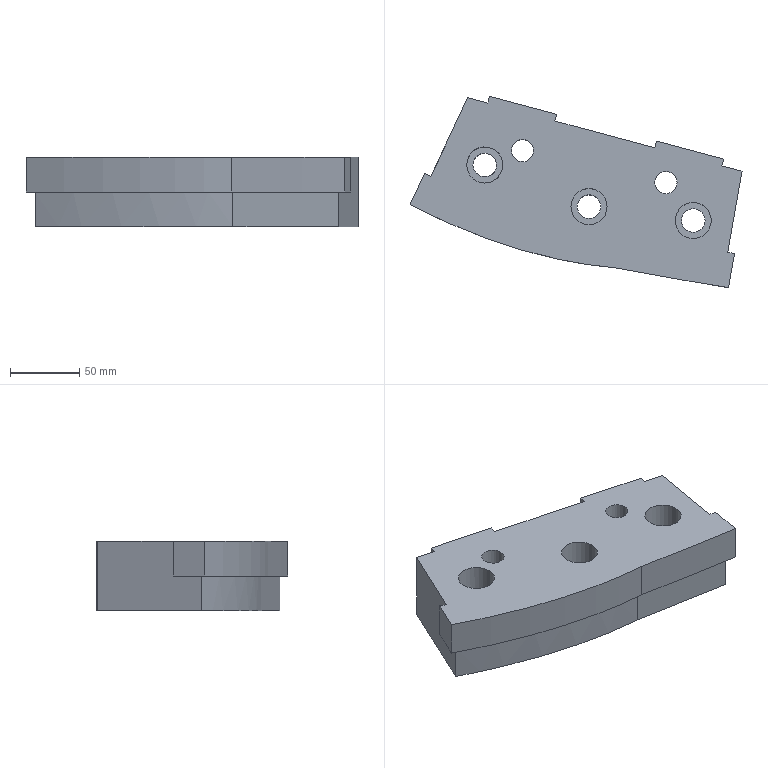Part | NX | features solid 2 | 1 solid | 33 faces | box 238.954 x 137.716 x 50 mm | volume 914448 mm3 | plane 21 | cylinder 8 | spline 4 | commonest cylinder face diameters 17 x3 26 x3 16 x2
STEP:
#1=CARTESIAN_POINT('',(-391.104,-138.3,0.));
#2=VERTEX_POINT('',#1);
#3=CARTESIAN_POINT('',(-376.615,-142.182,0.));
#4=VERTEX_POINT('',#3);
#5=CARTESIAN_POINT('',(-578.987,-87.957,0.));
#6=DIRECTION('',(0.9659,-0.2588,0.));
#7=VECTOR('',#6,1000.);
#8=LINE('',#5,#7);
#9=EDGE_CURVE('',#2,#4,#8,.T.);
#10=ORIENTED_EDGE('',*,*,#9,.T.);
#11=CARTESIAN_POINT('',(-376.615,-142.182,-50.));
#12=VERTEX_POINT('',#11);
#13=CARTESIAN_POINT('',(-376.615,-142.182,-50.));
#14=DIRECTION('',(0.,0.,-1.));
#15=VECTOR('',#14,1000.);
#16=LINE('',#13,#15);
#17=EDGE_CURVE('',#4,#12,#16,.T.);
#18=ORIENTED_EDGE('',*,*,#17,.T.);
#19=CARTESIAN_POINT('',(-391.104,-138.3,-50.));
#20=VERTEX_POINT('',#19);
#21=CARTESIAN_POINT('',(-578.987,-87.957,-50.));
#22=DIRECTION('',(0.9659,-0.2588,0.));
#23=VECTOR('',#22,1000.);
#24=LINE('',#21,#23);
#25=EDGE_CURVE('',#20,#12,#24,.T.);
#26=ORIENTED_EDGE('',*,*,#25,.F.);
#27=CARTESIAN_POINT('',(-391.104,-138.3,-50.));
#28=DIRECTION('',(0.,0.,1.));
#29=VECTOR('',#28,1000.);
#30=LINE('',#27,#29);
#31=EDGE_CURVE('',#20,#2,#30,.T.);
#32=ORIENTED_EDGE('',*,*,#31,.T.);
#33=EDGE_LOOP('',(#10,#18,#26,#32));
#34=FACE_BOUND('',#33,.T.);
#35=CARTESIAN_POINT('',(-578.987,-87.957,-50.));
#36=DIRECTION('',(-0.2588,-0.9659,0.));
#37=DIRECTION('',(0.9659,-0.2588,0.));
#38=AXIS2_PLACEMENT_3D('',#35,#36,#37);
#39=PLANE('',#38);
#40=ADVANCED_FACE('',(#34),#39,.F.);
#41=CARTESIAN_POINT('',(-381.983,-201.42,-25.));
#42=VERTEX_POINT('',#41);
#43=CARTESIAN_POINT('',(-386.907,-200.551,-25.));
#44=VERTEX_POINT('',#43);
#45=CARTESIAN_POINT('',(-377.059,-202.288,-25.));
#46=DIRECTION('',(-0.9848,0.1736,0.));
#47=VECTOR('',#46,1000.);
#48=LINE('',#45,#47);
#49=EDGE_CURVE('',#42,#44,#48,.T.);
#50=ORIENTED_EDGE('',*,*,#49,.F.);
#51=CARTESIAN_POINT('',(-386.325,-226.04,-25.));
#52=VERTEX_POINT('',#51);
#53=CARTESIAN_POINT('',(-386.325,-226.04,-25.));
#54=DIRECTION('',(-0.1736,-0.9848,0.));
#55=VECTOR('',#54,1000.);
#56=LINE('',#53,#55);
#57=EDGE_CURVE('',#42,#52,#56,.T.);
#58=ORIENTED_EDGE('',*,*,#57,.T.);
#59=CARTESIAN_POINT('',(-467.332,-211.778,-25.));
#60=VERTEX_POINT('',#59);
#61=CARTESIAN_POINT('',(-467.332,-211.778,-25.));
#62=CARTESIAN_POINT('',(-453.683,-214.296,-25.));
#63=CARTESIAN_POINT('',(-426.719,-219.268,-25.));
#64=CARTESIAN_POINT('',(-399.705,-223.975,-25.));
#65=CARTESIAN_POINT('',(-386.325,-226.04,-25.));
#66=B_SPLINE_CURVE_WITH_KNOTS('',3,(#61,#62,#63,#64,#65),.UNSPECIFIED.,.F.,.F.,(4,1,4),(0.6548,0.8295,1.),.UNSPECIFIED.);
#67=EDGE_CURVE('',#52,#60,#66,.F.);
#68=ORIENTED_EDGE('',*,*,#67,.T.);
#69=CARTESIAN_POINT('',(-615.57,-166.409,-25.));
#70=VERTEX_POINT('',#69);
#71=CARTESIAN_POINT('',(-615.57,-166.409,-25.));
#72=CARTESIAN_POINT('',(-612.933,-167.769,-25.));
#73=CARTESIAN_POINT('',(-595.69,-176.474,-25.));
#74=CARTESIAN_POINT('',(-562.946,-190.715,-25.));
#75=CARTESIAN_POINT('',(-515.99,-205.204,-25.));
#76=CARTESIAN_POINT('',(-483.626,-210.452,-25.));
#77=CARTESIAN_POINT('',(-467.332,-211.778,-25.));
#78=B_SPLINE_CURVE_WITH_KNOTS('',3,(#71,#72,#73,#74,#75,#76,#77),.UNSPECIFIED.,.F.,.F.,(4,1,1,1,4),(0.,0.03735,0.2432,0.449,0.6548),.UNSPECIFIED.);
#79=EDGE_CURVE('',#60,#70,#78,.F.);
#80=ORIENTED_EDGE('',*,*,#79,.T.);
#81=CARTESIAN_POINT('',(-605.004,-143.752,-25.));
#82=VERTEX_POINT('',#81);
#83=CARTESIAN_POINT('',(-615.57,-166.409,-25.));
#84=DIRECTION('',(-0.4226,-0.9063,0.));
#85=VECTOR('',#84,1000.);
#86=LINE('',#83,#85);
#87=EDGE_CURVE('',#82,#70,#86,.T.);
#88=ORIENTED_EDGE('',*,*,#87,.F.);
#89=CARTESIAN_POINT('',(-600.473,-145.865,-25.));
#90=VERTEX_POINT('',#89);
#91=CARTESIAN_POINT('',(-609.536,-141.638,-25.));
#92=DIRECTION('',(0.9063,-0.4226,0.));
#93=VECTOR('',#92,1000.);
#94=LINE('',#91,#93);
#95=EDGE_CURVE('',#82,#90,#94,.T.);
#96=ORIENTED_EDGE('',*,*,#95,.T.);
#97=CARTESIAN_POINT('',(-608.998,-164.148,-25.));
#98=VERTEX_POINT('',#97);
#99=CARTESIAN_POINT('',(-611.038,-168.522,-25.));
#100=DIRECTION('',(-0.4226,-0.9063,0.));
#101=VECTOR('',#100,1000.);
#102=LINE('',#99,#101);
#103=EDGE_CURVE('',#98,#90,#102,.F.);
#104=ORIENTED_EDGE('',*,*,#103,.F.);
#105=CARTESIAN_POINT('',(-466.674,-206.815,-25.));
#106=VERTEX_POINT('',#105);
#107=CARTESIAN_POINT('',(-608.998,-164.148,-25.));
#108=CARTESIAN_POINT('',(-597.84,-169.769,-25.));
#109=CARTESIAN_POINT('',(-575.112,-180.178,-25.));
#110=CARTESIAN_POINT('',(-545.758,-190.822,-25.));
#111=CARTESIAN_POINT('',(-521.796,-197.632,-25.));
#112=CARTESIAN_POINT('',(-503.595,-201.793,-25.));
#113=CARTESIAN_POINT('',(-488.289,-204.412,-25.));
#114=CARTESIAN_POINT('',(-475.931,-205.974,-25.));
#115=CARTESIAN_POINT('',(-469.818,-206.559,-25.));
#116=CARTESIAN_POINT('',(-466.674,-206.815,-25.));
#117=B_SPLINE_CURVE_WITH_KNOTS('',3,(#107,#108,#109,#110,#111,#112,#113,#114,#115,#116),.UNSPECIFIED.,.F.,.F.,(4,1,1,1,1,1,1,4),(0.03109,0.2737,0.5164,0.6377,0.759,0.8803,0.941,1.002),.UNSPECIFIED.);
#118=EDGE_CURVE('',#98,#106,#117,.T.);
#119=ORIENTED_EDGE('',*,*,#118,.T.);
#120=CARTESIAN_POINT('',(-390.397,-220.341,-25.));
#121=VERTEX_POINT('',#120);
#122=CARTESIAN_POINT('',(-466.674,-206.815,-25.));
#123=CARTESIAN_POINT('',(-453.956,-209.161,-25.));
#124=CARTESIAN_POINT('',(-428.53,-213.847,-25.));
#125=CARTESIAN_POINT('',(-403.113,-218.32,-25.));
#126=CARTESIAN_POINT('',(-390.397,-220.341,-25.));
#127=B_SPLINE_CURVE_WITH_KNOTS('',3,(#122,#123,#124,#125,#126),.UNSPECIFIED.,.F.,.F.,(4,1,4),(-0.003079,0.4686,0.9402),.UNSPECIFIED.);
#128=EDGE_CURVE('',#106,#121,#127,.T.);
#129=ORIENTED_EDGE('',*,*,#128,.T.);
#130=CARTESIAN_POINT('',(-391.249,-225.172,-25.));
#131=DIRECTION('',(-0.1736,-0.9848,0.));
#132=VECTOR('',#131,1000.);
#133=LINE('',#130,#132);
#134=EDGE_CURVE('',#121,#44,#133,.F.);
#135=ORIENTED_EDGE('',*,*,#134,.T.);
#136=EDGE_LOOP('',(#50,#58,#68,#80,#88,#96,#104,#119,#129,#135));
#137=FACE_BOUND('',#136,.T.);
#138=CARTESIAN_POINT('',(-280.448,-255.656,-25.));
#139=DIRECTION('',(0.,0.,-1.));
#140=DIRECTION('',(-1.,0.,0.));
#141=AXIS2_PLACEMENT_3D('',#138,#139,#140);
#142=PLANE('',#141);
#143=ADVANCED_FACE('',(#137),#142,.T.);
#144=CARTESIAN_POINT('',(-526.523,-127.421,0.));
#145=VERTEX_POINT('',#144);
#146=CARTESIAN_POINT('',(-534.523,-127.421,0.));
#147=DIRECTION('',(0.,0.,1.));
#148=DIRECTION('',(1.,0.,0.));
#149=AXIS2_PLACEMENT_3D('',#146,#147,#148);
#150=CIRCLE('',#149,8.);
#151=EDGE_CURVE('',#145,#145,#150,.T.);
#152=ORIENTED_EDGE('',*,*,#151,.F.);
#153=EDGE_LOOP('',(#152));
#154=FACE_BOUND('',#153,.T.);
#155=CARTESIAN_POINT('',(-423.374,-150.368,0.));
#156=VERTEX_POINT('',#155);
#157=CARTESIAN_POINT('',(-431.374,-150.368,0.));
#158=DIRECTION('',(0.,0.,1.));
#159=DIRECTION('',(1.,0.,0.));
#160=AXIS2_PLACEMENT_3D('',#157,#158,#159);
#161=CIRCLE('',#160,8.);
#162=EDGE_CURVE('',#156,#156,#161,.T.);
#163=ORIENTED_EDGE('',*,*,#162,.F.);
#164=EDGE_LOOP('',(#163));
#165=FACE_BOUND('',#164,.T.);
#166=CARTESIAN_POINT('',(-381.983,-201.42,0.));
#167=VERTEX_POINT('',#166);
#168=CARTESIAN_POINT('',(-386.907,-200.551,0.));
#169=VERTEX_POINT('',#168);
#170=CARTESIAN_POINT('',(-377.059,-202.288,0.));
#171=DIRECTION('',(-0.9848,0.1736,0.));
#172=VECTOR('',#171,1000.);
#173=LINE('',#170,#172);
#174=EDGE_CURVE('',#167,#169,#173,.T.);
#175=ORIENTED_EDGE('',*,*,#174,.T.);
#176=CARTESIAN_POINT('',(-391.249,-225.172,0.));
#177=DIRECTION('',(0.1736,0.9848,0.));
#178=VECTOR('',#177,1000.);
#179=LINE('',#176,#178);
#180=EDGE_CURVE('',#169,#4,#179,.T.);
#181=ORIENTED_EDGE('',*,*,#180,.T.);
#182=ORIENTED_EDGE('',*,*,#9,.F.);
#183=CARTESIAN_POINT('',(-389.81,-133.47,0.));
#184=VERTEX_POINT('',#183);
#185=CARTESIAN_POINT('',(-391.104,-138.3,0.));
#186=DIRECTION('',(0.2588,0.9659,0.));
#187=VECTOR('',#186,1000.);
#188=LINE('',#185,#187);
#189=EDGE_CURVE('',#2,#184,#188,.T.);
#190=ORIENTED_EDGE('',*,*,#189,.T.);
#191=CARTESIAN_POINT('',(-438.106,-120.529,0.));
#192=VERTEX_POINT('',#191);
#193=CARTESIAN_POINT('',(-577.693,-83.127,0.));
#194=DIRECTION('',(0.9659,-0.2588,0.));
#195=VECTOR('',#194,1000.);
#196=LINE('',#193,#195);
#197=EDGE_CURVE('',#192,#184,#196,.T.);
#198=ORIENTED_EDGE('',*,*,#197,.F.);
#199=CARTESIAN_POINT('',(-439.401,-125.359,0.));
#200=VERTEX_POINT('',#199);
#201=CARTESIAN_POINT('',(-439.401,-125.359,0.));
#202=DIRECTION('',(0.2588,0.9659,0.));
#203=VECTOR('',#202,1000.);
#204=LINE('',#201,#203);
#205=EDGE_CURVE('',#200,#192,#204,.T.);
#206=ORIENTED_EDGE('',*,*,#205,.F.);
#207=CARTESIAN_POINT('',(-511.297,-106.094,0.));
#208=VERTEX_POINT('',#207);
#209=CARTESIAN_POINT('',(-578.987,-87.957,0.));
#210=DIRECTION('',(0.9659,-0.2588,0.));
#211=VECTOR('',#210,1000.);
#212=LINE('',#209,#211);
#213=EDGE_CURVE('',#208,#200,#212,.T.);
#214=ORIENTED_EDGE('',*,*,#213,.F.);
#215=CARTESIAN_POINT('',(-510.003,-101.265,0.));
#216=VERTEX_POINT('',#215);
#217=CARTESIAN_POINT('',(-511.297,-106.094,0.));
#218=DIRECTION('',(0.2588,0.9659,0.));
#219=VECTOR('',#218,1000.);
#220=LINE('',#217,#219);
#221=EDGE_CURVE('',#208,#216,#220,.T.);
#222=ORIENTED_EDGE('',*,*,#221,.T.);
#223=CARTESIAN_POINT('',(-558.3,-88.324,0.));
#224=VERTEX_POINT('',#223);
#225=CARTESIAN_POINT('',(-712.375,-47.039,0.));
#226=DIRECTION('',(0.9659,-0.2588,0.));
#227=VECTOR('',#226,1000.);
#228=LINE('',#225,#227);
#229=EDGE_CURVE('',#224,#216,#228,.T.);
#230=ORIENTED_EDGE('',*,*,#229,.F.);
#231=CARTESIAN_POINT('',(-559.594,-93.153,0.));
#232=VERTEX_POINT('',#231);
#233=CARTESIAN_POINT('',(-559.594,-93.153,0.));
#234=DIRECTION('',(0.2588,0.9659,0.));
#235=VECTOR('',#234,1000.);
#236=LINE('',#233,#235);
#237=EDGE_CURVE('',#232,#224,#236,.T.);
#238=ORIENTED_EDGE('',*,*,#237,.F.);
#239=CARTESIAN_POINT('',(-574.083,-89.271,0.));
#240=VERTEX_POINT('',#239);
#241=CARTESIAN_POINT('',(-578.987,-87.957,0.));
#242=DIRECTION('',(0.9659,-0.2588,0.));
#243=VECTOR('',#242,1000.);
#244=LINE('',#241,#243);
#245=EDGE_CURVE('',#240,#232,#244,.T.);
#246=ORIENTED_EDGE('',*,*,#245,.F.);
#247=CARTESIAN_POINT('',(-600.473,-145.865,0.));
#248=VERTEX_POINT('',#247);
#249=CARTESIAN_POINT('',(-611.038,-168.522,0.));
#250=DIRECTION('',(0.4226,0.9063,0.));
#251=VECTOR('',#250,1000.);
#252=LINE('',#249,#251);
#253=EDGE_CURVE('',#248,#240,#252,.T.);
#254=ORIENTED_EDGE('',*,*,#253,.F.);
#255=CARTESIAN_POINT('',(-605.004,-143.752,0.));
#256=VERTEX_POINT('',#255);
#257=CARTESIAN_POINT('',(-609.536,-141.638,0.));
#258=DIRECTION('',(0.9063,-0.4226,0.));
#259=VECTOR('',#258,1000.);
#260=LINE('',#257,#259);
#261=EDGE_CURVE('',#256,#248,#260,.T.);
#262=ORIENTED_EDGE('',*,*,#261,.F.);
#263=CARTESIAN_POINT('',(-615.57,-166.409,0.));
#264=VERTEX_POINT('',#263);
#265=CARTESIAN_POINT('',(-615.57,-166.409,0.));
#266=DIRECTION('',(0.4226,0.9063,0.));
#267=VECTOR('',#266,1000.);
#268=LINE('',#265,#267);
#269=EDGE_CURVE('',#264,#256,#268,.T.);
#270=ORIENTED_EDGE('',*,*,#269,.F.);
#271=CARTESIAN_POINT('',(-467.332,-211.778,0.));
#272=VERTEX_POINT('',#271);
#273=CARTESIAN_POINT('',(-615.57,-166.409,0.));
#274=CARTESIAN_POINT('',(-612.933,-167.769,0.));
#275=CARTESIAN_POINT('',(-595.69,-176.474,0.));
#276=CARTESIAN_POINT('',(-562.946,-190.715,0.));
#277=CARTESIAN_POINT('',(-515.99,-205.204,0.));
#278=CARTESIAN_POINT('',(-483.626,-210.452,0.));
#279=CARTESIAN_POINT('',(-467.332,-211.778,0.));
#280=B_SPLINE_CURVE_WITH_KNOTS('',3,(#273,#274,#275,#276,#277,#278,#279),.UNSPECIFIED.,.F.,.F.,(4,1,1,1,4),(0.,0.03735,0.2432,0.449,0.6548),.UNSPECIFIED.);
#281=EDGE_CURVE('',#264,#272,#280,.T.);
#282=ORIENTED_EDGE('',*,*,#281,.T.);
#283=CARTESIAN_POINT('',(-386.325,-226.04,0.));
#284=VERTEX_POINT('',#283);
#285=CARTESIAN_POINT('',(-467.332,-211.778,0.));
#286=CARTESIAN_POINT('',(-453.683,-214.296,0.));
#287=CARTESIAN_POINT('',(-426.719,-219.268,0.));
#288=CARTESIAN_POINT('',(-399.705,-223.975,0.));
#289=CARTESIAN_POINT('',(-386.325,-226.04,0.));
#290=B_SPLINE_CURVE_WITH_KNOTS('',3,(#285,#286,#287,#288,#289),.UNSPECIFIED.,.F.,.F.,(4,1,4),(0.6548,0.8295,1.),.UNSPECIFIED.);
#291=EDGE_CURVE('',#272,#284,#290,.T.);
#292=ORIENTED_EDGE('',*,*,#291,.T.);
#293=CARTESIAN_POINT('',(-386.325,-226.04,0.));
#294=DIRECTION('',(0.1736,0.9848,0.));
#295=VECTOR('',#294,1000.);
#296=LINE('',#293,#295);
#297=EDGE_CURVE('',#284,#167,#296,.T.);
#298=ORIENTED_EDGE('',*,*,#297,.T.);
#299=EDGE_LOOP('',(#175,#181,#182,#190,#198,#206,#214,#222,#230,#238,#246,#254,#262,#270,#282,#292,#298));
#300=FACE_BOUND('',#299,.T.);
#301=CARTESIAN_POINT('',(-574.729,-137.741,0.));
#302=VERTEX_POINT('',#301);
#303=CARTESIAN_POINT('',(-561.729,-137.741,0.));
#304=DIRECTION('',(0.,0.,-1.));
#305=DIRECTION('',(-1.,0.,0.));
#306=AXIS2_PLACEMENT_3D('',#303,#304,#305);
#307=CIRCLE('',#306,13.);
#308=EDGE_CURVE('',#302,#302,#307,.T.);
#309=ORIENTED_EDGE('',*,*,#308,.T.);
#310=EDGE_LOOP('',(#309));
#311=FACE_BOUND('',#310,.T.);
#312=CARTESIAN_POINT('',(-499.729,-167.741,0.));
#313=VERTEX_POINT('',#312);
#314=CARTESIAN_POINT('',(-486.729,-167.741,0.));
#315=DIRECTION('',(0.,0.,-1.));
#316=DIRECTION('',(-1.,0.,0.));
#317=AXIS2_PLACEMENT_3D('',#314,#315,#316);
#318=CIRCLE('',#317,13.);
#319=EDGE_CURVE('',#313,#313,#318,.T.);
#320=ORIENTED_EDGE('',*,*,#319,.T.);
#321=EDGE_LOOP('',(#320));
#322=FACE_BOUND('',#321,.T.);
#323=CARTESIAN_POINT('',(-424.729,-177.741,0.));
#324=VERTEX_POINT('',#323);
#325=CARTESIAN_POINT('',(-411.729,-177.741,0.));
#326=DIRECTION('',(0.,0.,-1.));
#327=DIRECTION('',(-1.,0.,0.));
#328=AXIS2_PLACEMENT_3D('',#325,#326,#327);
#329=CIRCLE('',#328,13.);
#330=EDGE_CURVE('',#324,#324,#329,.T.);
#331=ORIENTED_EDGE('',*,*,#330,.T.);
#332=EDGE_LOOP('',(#331));
#333=FACE_BOUND('',#332,.T.);
#334=CARTESIAN_POINT('',(-488.834,-961.671,0.));
#335=DIRECTION('',(0.,0.,1.));
#336=DIRECTION('',(1.,0.,0.));
#337=AXIS2_PLACEMENT_3D('',#334,#335,#336);
#338=PLANE('',#337);
#339=ADVANCED_FACE('',(#154,#165,#300,#311,#322,#333),#338,.T.);
#340=CARTESIAN_POINT('',(-605.004,-143.752,-50.));
#341=DIRECTION('',(0.,0.,1.));
#342=VECTOR('',#341,1000.);
#343=LINE('',#340,#342);
#344=EDGE_CURVE('',#82,#256,#343,.T.);
#345=ORIENTED_EDGE('',*,*,#344,.F.);
#346=ORIENTED_EDGE('',*,*,#87,.T.);
#347=CARTESIAN_POINT('',(-615.57,-166.409,-50.));
#348=DIRECTION('',(0.,0.,1.));
#349=VECTOR('',#348,1000.);
#350=LINE('',#347,#349);
#351=EDGE_CURVE('',#70,#264,#350,.T.);
#352=ORIENTED_EDGE('',*,*,#351,.T.);
#353=ORIENTED_EDGE('',*,*,#269,.T.);
#354=EDGE_LOOP('',(#345,#346,#352,#353));
#355=FACE_BOUND('',#354,.T.);
#356=CARTESIAN_POINT('',(-615.57,-166.409,-50.));
#357=DIRECTION('',(0.9063,-0.4226,0.));
#358=DIRECTION('',(0.4226,0.9063,0.));
#359=AXIS2_PLACEMENT_3D('',#356,#357,#358);
#360=PLANE('',#359);
#361=ADVANCED_FACE('',(#355),#360,.F.);
#362=CARTESIAN_POINT('',(-526.523,-127.421,-50.));
#363=VERTEX_POINT('',#362);
#364=CARTESIAN_POINT('',(-534.523,-127.421,-50.));
#365=DIRECTION('',(0.,0.,1.));
#366=DIRECTION('',(1.,0.,0.));
#367=AXIS2_PLACEMENT_3D('',#364,#365,#366);
#368=CIRCLE('',#367,8.);
#369=EDGE_CURVE('',#363,#363,#368,.T.);
#370=ORIENTED_EDGE('',*,*,#369,.T.);
#371=EDGE_LOOP('',(#370));
#372=FACE_BOUND('',#371,.T.);
#373=CARTESIAN_POINT('',(-423.374,-150.368,-50.));
#374=VERTEX_POINT('',#373);
#375=CARTESIAN_POINT('',(-431.374,-150.368,-50.));
#376=DIRECTION('',(0.,0.,1.));
#377=DIRECTION('',(1.,0.,0.));
#378=AXIS2_PLACEMENT_3D('',#375,#376,#377);
#379=CIRCLE('',#378,8.);
#380=EDGE_CURVE('',#374,#374,#379,.T.);
#381=ORIENTED_EDGE('',*,*,#380,.T.);
#382=EDGE_LOOP('',(#381));
#383=FACE_BOUND('',#382,.T.);
#384=ORIENTED_EDGE('',*,*,#25,.T.);
#385=CARTESIAN_POINT('',(-390.397,-220.341,-50.));
#386=VERTEX_POINT('',#385);
#387=CARTESIAN_POINT('',(-391.297,-225.445,-50.));
#388=DIRECTION('',(0.1736,0.9848,0.));
#389=VECTOR('',#388,1000.);
#390=LINE('',#387,#389);
#391=EDGE_CURVE('',#386,#12,#390,.T.);
#392=ORIENTED_EDGE('',*,*,#391,.F.);
#393=CARTESIAN_POINT('',(-466.674,-206.815,-50.));
#394=VERTEX_POINT('',#393);
#395=CARTESIAN_POINT('',(-390.397,-220.341,-50.));
#396=CARTESIAN_POINT('',(-392.903,-219.943,-50.));
#397=CARTESIAN_POINT('',(-396.916,-219.29,-50.));
#398=CARTESIAN_POINT('',(-402.772,-218.308,-50.));
#399=CARTESIAN_POINT('',(-407.418,-217.517,-50.));
#400=CARTESIAN_POINT('',(-412.316,-216.67,-50.));
#401=CARTESIAN_POINT('',(-416.609,-215.918,-50.));
#402=CARTESIAN_POINT('',(-420.17,-215.288,-50.));
#403=CARTESIAN_POINT('',(-422.448,-214.883,-50.));
#404=CARTESIAN_POINT('',(-424.302,-214.553,-50.));
#405=CARTESIAN_POINT('',(-425.71,-214.301,-50.));
#406=CARTESIAN_POINT('',(-426.889,-214.089,-50.));
#407=CARTESIAN_POINT('',(-427.737,-213.937,-50.));
#408=CARTESIAN_POINT('',(-428.198,-213.854,-50.));
#409=CARTESIAN_POINT('',(-428.618,-213.778,-50.));
#410=CARTESIAN_POINT('',(-428.759,-213.753,-50.));
#411=CARTESIAN_POINT('',(-429.048,-213.701,-50.));
#412=CARTESIAN_POINT('',(-429.513,-213.617,-50.));
#413=CARTESIAN_POINT('',(-430.215,-213.49,-50.));
#414=CARTESIAN_POINT('',(-431.073,-213.335,-50.));
#415=CARTESIAN_POINT('',(-432.253,-213.122,-50.));
#416=CARTESIAN_POINT('',(-433.788,-212.844,-50.));
#417=CARTESIAN_POINT('',(-436.376,-212.374,-50.));
#418=CARTESIAN_POINT('',(-439.855,-211.74,-50.));
#419=CARTESIAN_POINT('',(-444.421,-210.906,-50.));
#420=CARTESIAN_POINT('',(-449.38,-209.997,-50.));
#421=CARTESIAN_POINT('',(-456.515,-208.687,-50.));
#422=CARTESIAN_POINT('',(-462.453,-207.593,-50.));
#423=CARTESIAN_POINT('',(-466.674,-206.815,-50.));
#424=B_SPLINE_CURVE_WITH_KNOTS('',3,(#395,#396,#397,#398,#399,#400,#401,#402,#403,#404,#405,#406,#407,#408,#409,#410,#411,#412,#413,#414,#415,#416,#417,#418,#419,#420,#421,#422,#423),.UNSPECIFIED.,.F.,.F.,(4,1,1,1,1,1,1,1,1,1,1,1,1,1,1,1,1,1,1,1,1,1,1,1,1,1,4),(0.,0.125,0.1875,0.25,0.3125,0.375,0.4062,0.4375,0.4531,0.4688,0.4844,0.4922,0.4961,0.5,0.5039,0.5078,0.5156,0.5312,0.5469,0.5625,0.5938,0.625,0.6875,0.75,0.8125,0.875,1.),.UNSPECIFIED.);
#425=EDGE_CURVE('',#394,#386,#424,.F.);
#426=ORIENTED_EDGE('',*,*,#425,.F.);
#427=CARTESIAN_POINT('',(-608.998,-164.148,-50.));
#428=VERTEX_POINT('',#427);
#429=CARTESIAN_POINT('',(-466.674,-206.815,-50.));
#430=CARTESIAN_POINT('',(-472.665,-206.327,-50.));
#431=CARTESIAN_POINT('',(-484.698,-204.994,-50.));
#432=CARTESIAN_POINT('',(-499.862,-202.433,-50.));
#433=CARTESIAN_POINT('',(-512.066,-199.847,-50.));
#434=CARTESIAN_POINT('',(-521.259,-197.639,-50.));
#435=CARTESIAN_POINT('',(-528.941,-195.578,-50.));
#436=CARTESIAN_POINT('',(-534.353,-194.012,-50.));
#437=CARTESIAN_POINT('',(-537.422,-193.092,-50.));
#438=CARTESIAN_POINT('',(-539.804,-192.361,-50.));
#439=CARTESIAN_POINT('',(-541.892,-191.707,-50.));
#440=CARTESIAN_POINT('',(-544.779,-190.785,-50.));
#441=CARTESIAN_POINT('',(-549.787,-189.14,-50.));
#442=CARTESIAN_POINT('',(-556.976,-186.647,-50.));
#443=CARTESIAN_POINT('',(-565.606,-183.442,-50.));
#444=CARTESIAN_POINT('',(-577.137,-178.882,-50.));
#445=CARTESIAN_POINT('',(-591.588,-172.642,-50.));
#446=CARTESIAN_POINT('',(-603.188,-167.075,-50.));
#447=CARTESIAN_POINT('',(-608.998,-164.148,-50.));
#448=B_SPLINE_CURVE_WITH_KNOTS('',3,(#429,#430,#431,#432,#433,#434,#435,#436,#437,#438,#439,#440,#441,#442,#443,#444,#445,#446,#447),.UNSPECIFIED.,.F.,.F.,(4,1,1,1,1,1,1,1,1,1,1,1,1,1,1,1,4),(0.,0.125,0.25,0.3125,0.375,0.4375,0.4688,0.4844,0.5,0.5156,0.5312,0.5625,0.625,0.6875,0.75,0.875,1.),.UNSPECIFIED.);
#449=EDGE_CURVE('',#428,#394,#448,.F.);
#450=ORIENTED_EDGE('',*,*,#449,.F.);
#451=CARTESIAN_POINT('',(-574.083,-89.271,-50.));
#452=VERTEX_POINT('',#451);
#453=CARTESIAN_POINT('',(-597.545,-139.587,-50.));
#454=DIRECTION('',(0.4226,0.9063,0.));
#455=VECTOR('',#454,1000.);
#456=LINE('',#453,#455);
#457=EDGE_CURVE('',#428,#452,#456,.T.);
#458=ORIENTED_EDGE('',*,*,#457,.T.);
#459=CARTESIAN_POINT('',(-559.594,-93.153,-50.));
#460=VERTEX_POINT('',#459);
#461=CARTESIAN_POINT('',(-578.987,-87.957,-50.));
#462=DIRECTION('',(0.9659,-0.2588,0.));
#463=VECTOR('',#462,1000.);
#464=LINE('',#461,#463);
#465=EDGE_CURVE('',#452,#460,#464,.T.);
#466=ORIENTED_EDGE('',*,*,#465,.T.);
#467=CARTESIAN_POINT('',(-558.3,-88.324,-50.));
#468=VERTEX_POINT('',#467);
#469=CARTESIAN_POINT('',(-559.594,-93.153,-50.));
#470=DIRECTION('',(0.2588,0.9659,0.));
#471=VECTOR('',#470,1000.);
#472=LINE('',#469,#471);
#473=EDGE_CURVE('',#460,#468,#472,.T.);
#474=ORIENTED_EDGE('',*,*,#473,.T.);
#475=CARTESIAN_POINT('',(-510.003,-101.265,-50.));
#476=VERTEX_POINT('',#475);
#477=CARTESIAN_POINT('',(-712.375,-47.039,-50.));
#478=DIRECTION('',(0.9659,-0.2588,0.));
#479=VECTOR('',#478,1000.);
#480=LINE('',#477,#479);
#481=EDGE_CURVE('',#468,#476,#480,.T.);
#482=ORIENTED_EDGE('',*,*,#481,.T.);
#483=CARTESIAN_POINT('',(-511.297,-106.094,-50.));
#484=VERTEX_POINT('',#483);
#485=CARTESIAN_POINT('',(-511.297,-106.094,-50.));
#486=DIRECTION('',(0.2588,0.9659,0.));
#487=VECTOR('',#486,1000.);
#488=LINE('',#485,#487);
#489=EDGE_CURVE('',#484,#476,#488,.T.);
#490=ORIENTED_EDGE('',*,*,#489,.F.);
#491=CARTESIAN_POINT('',(-439.401,-125.359,-50.));
#492=VERTEX_POINT('',#491);
#493=CARTESIAN_POINT('',(-578.987,-87.957,-50.));
#494=DIRECTION('',(0.9659,-0.2588,0.));
#495=VECTOR('',#494,1000.);
#496=LINE('',#493,#495);
#497=EDGE_CURVE('',#484,#492,#496,.T.);
#498=ORIENTED_EDGE('',*,*,#497,.T.);
#499=CARTESIAN_POINT('',(-438.106,-120.529,-50.));
#500=VERTEX_POINT('',#499);
#501=CARTESIAN_POINT('',(-439.401,-125.359,-50.));
#502=DIRECTION('',(0.2588,0.9659,0.));
#503=VECTOR('',#502,1000.);
#504=LINE('',#501,#503);
#505=EDGE_CURVE('',#492,#500,#504,.T.);
#506=ORIENTED_EDGE('',*,*,#505,.T.);
#507=CARTESIAN_POINT('',(-389.81,-133.47,-50.));
#508=VERTEX_POINT('',#507);
#509=CARTESIAN_POINT('',(-577.693,-83.127,-50.));
#510=DIRECTION('',(0.9659,-0.2588,0.));
#511=VECTOR('',#510,1000.);
#512=LINE('',#509,#511);
#513=EDGE_CURVE('',#500,#508,#512,.T.);
#514=ORIENTED_EDGE('',*,*,#513,.T.);
#515=CARTESIAN_POINT('',(-391.104,-138.3,-50.));
#516=DIRECTION('',(0.2588,0.9659,0.));
#517=VECTOR('',#516,1000.);
#518=LINE('',#515,#517);
#519=EDGE_CURVE('',#20,#508,#518,.T.);
#520=ORIENTED_EDGE('',*,*,#519,.F.);
#521=EDGE_LOOP('',(#384,#392,#426,#450,#458,#466,#474,#482,#490,#498,#506,#514,#520));
#522=FACE_BOUND('',#521,.T.);
#523=CARTESIAN_POINT('',(-420.229,-177.741,-50.));
#524=VERTEX_POINT('',#523);
#525=CARTESIAN_POINT('',(-411.729,-177.741,-50.));
#526=DIRECTION('',(0.,0.,-1.));
#527=DIRECTION('',(-1.,0.,0.));
#528=AXIS2_PLACEMENT_3D('',#525,#526,#527);
#529=CIRCLE('',#528,8.5);
#530=EDGE_CURVE('',#524,#524,#529,.T.);
#531=ORIENTED_EDGE('',*,*,#530,.F.);
#532=EDGE_LOOP('',(#531));
#533=FACE_BOUND('',#532,.T.);
#534=CARTESIAN_POINT('',(-495.229,-167.741,-50.));
#535=VERTEX_POINT('',#534);
#536=CARTESIAN_POINT('',(-486.729,-167.741,-50.));
#537=DIRECTION('',(0.,0.,-1.));
#538=DIRECTION('',(-1.,0.,0.));
#539=AXIS2_PLACEMENT_3D('',#536,#537,#538);
#540=CIRCLE('',#539,8.5);
#541=EDGE_CURVE('',#535,#535,#540,.T.);
#542=ORIENTED_EDGE('',*,*,#541,.F.);
#543=EDGE_LOOP('',(#542));
#544=FACE_BOUND('',#543,.T.);
#545=CARTESIAN_POINT('',(-570.229,-137.741,-50.));
#546=VERTEX_POINT('',#545);
#547=CARTESIAN_POINT('',(-561.729,-137.741,-50.));
#548=DIRECTION('',(0.,0.,-1.));
#549=DIRECTION('',(-1.,0.,0.));
#550=AXIS2_PLACEMENT_3D('',#547,#548,#549);
#551=CIRCLE('',#550,8.5);
#552=EDGE_CURVE('',#546,#546,#551,.T.);
#553=ORIENTED_EDGE('',*,*,#552,.F.);
#554=EDGE_LOOP('',(#553));
#555=FACE_BOUND('',#554,.T.);
#556=CARTESIAN_POINT('',(-488.834,-961.671,-50.));
#557=DIRECTION('',(0.,0.,1.));
#558=DIRECTION('',(1.,0.,0.));
#559=AXIS2_PLACEMENT_3D('',#556,#557,#558);
#560=PLANE('',#559);
#561=ADVANCED_FACE('',(#372,#383,#522,#533,#544,#555),#560,.F.);
#562=CARTESIAN_POINT('',(-420.229,-177.741,-25.));
#563=VERTEX_POINT('',#562);
#564=CARTESIAN_POINT('',(-411.729,-177.741,-25.));
#565=DIRECTION('',(0.,0.,-1.));
#566=DIRECTION('',(-1.,0.,0.));
#567=AXIS2_PLACEMENT_3D('',#564,#565,#566);
#568=CIRCLE('',#567,8.5);
#569=EDGE_CURVE('',#563,#563,#568,.F.);
#570=ORIENTED_EDGE('',*,*,#569,.T.);
#571=EDGE_LOOP('',(#570));
#572=FACE_BOUND('',#571,.T.);
#573=ORIENTED_EDGE('',*,*,#530,.T.);
#574=EDGE_LOOP('',(#573));
#575=FACE_BOUND('',#574,.T.);
#576=CARTESIAN_POINT('',(-411.729,-177.741,-75.));
#577=DIRECTION('',(0.,0.,1.));
#578=DIRECTION('',(1.,0.,0.));
#579=AXIS2_PLACEMENT_3D('',#576,#577,#578);
#580=CYLINDRICAL_SURFACE('',#579,8.5);
#581=ADVANCED_FACE('',(#572,#575),#580,.F.);
#582=ORIENTED_EDGE('',*,*,#569,.F.);
#583=EDGE_LOOP('',(#582));
#584=FACE_BOUND('',#583,.T.);
#585=CARTESIAN_POINT('',(-398.729,-177.741,-25.));
#586=VERTEX_POINT('',#585);
#587=CARTESIAN_POINT('',(-411.729,-177.741,-25.));
#588=DIRECTION('',(0.,0.,1.));
#589=DIRECTION('',(1.,0.,0.));
#590=AXIS2_PLACEMENT_3D('',#587,#588,#589);
#591=CIRCLE('',#590,13.);
#592=EDGE_CURVE('',#586,#586,#591,.T.);
#593=ORIENTED_EDGE('',*,*,#592,.T.);
#594=EDGE_LOOP('',(#593));
#595=FACE_BOUND('',#594,.T.);
#596=CARTESIAN_POINT('',(-411.729,-177.741,-25.));
#597=DIRECTION('',(0.,0.,-1.));
#598=DIRECTION('',(-1.,0.,0.));
#599=AXIS2_PLACEMENT_3D('',#596,#597,#598);
#600=PLANE('',#599);
#601=ADVANCED_FACE('',(#584,#595),#600,.F.);
#602=ORIENTED_EDGE('',*,*,#330,.F.);
#603=EDGE_LOOP('',(#602));
#604=FACE_BOUND('',#603,.T.);
#605=ORIENTED_EDGE('',*,*,#592,.F.);
#606=EDGE_LOOP('',(#605));
#607=FACE_BOUND('',#606,.T.);
#608=CARTESIAN_POINT('',(-411.729,-177.741,-25.));
#609=DIRECTION('',(0.,0.,1.));
#610=DIRECTION('',(1.,0.,0.));
#611=AXIS2_PLACEMENT_3D('',#608,#609,#610);
#612=CYLINDRICAL_SURFACE('',#611,13.);
#613=ADVANCED_FACE('',(#604,#607),#612,.F.);
#614=ORIENTED_EDGE('',*,*,#118,.F.);
#615=CARTESIAN_POINT('',(-608.998,-164.148,-37.5));
#616=DIRECTION('',(0.,0.,-1.));
#617=VECTOR('',#616,1000.);
#618=LINE('',#615,#617);
#619=EDGE_CURVE('',#428,#98,#618,.F.);
#620=ORIENTED_EDGE('',*,*,#619,.F.);
#621=ORIENTED_EDGE('',*,*,#449,.T.);
#622=CARTESIAN_POINT('',(-466.674,-206.815,-42.5));
#623=DIRECTION('',(0.,0.,-1.));
#624=VECTOR('',#623,1000.);
#625=LINE('',#622,#624);
#626=EDGE_CURVE('',#106,#394,#625,.T.);
#627=ORIENTED_EDGE('',*,*,#626,.F.);
#628=EDGE_LOOP('',(#614,#620,#621,#627));
#629=FACE_BOUND('',#628,.T.);
#630=CARTESIAN_POINT('',(-608.998,-164.148,-25.));
#631=CARTESIAN_POINT('',(-608.998,-164.148,-50.));
#632=CARTESIAN_POINT('',(-597.84,-169.769,-25.));
#633=CARTESIAN_POINT('',(-597.84,-169.769,-50.));
#634=CARTESIAN_POINT('',(-575.112,-180.178,-25.));
#635=CARTESIAN_POINT('',(-575.112,-180.178,-50.));
#636=CARTESIAN_POINT('',(-545.758,-190.822,-25.));
#637=CARTESIAN_POINT('',(-545.758,-190.822,-50.));
#638=CARTESIAN_POINT('',(-521.796,-197.632,-25.));
#639=CARTESIAN_POINT('',(-521.796,-197.632,-50.));
#640=CARTESIAN_POINT('',(-503.595,-201.793,-25.));
#641=CARTESIAN_POINT('',(-503.595,-201.793,-50.));
#642=CARTESIAN_POINT('',(-488.289,-204.412,-25.));
#643=CARTESIAN_POINT('',(-488.289,-204.412,-50.));
#644=CARTESIAN_POINT('',(-475.931,-205.974,-25.));
#645=CARTESIAN_POINT('',(-475.931,-205.974,-50.));
#646=CARTESIAN_POINT('',(-469.818,-206.559,-25.));
#647=CARTESIAN_POINT('',(-469.818,-206.559,-50.));
#648=CARTESIAN_POINT('',(-466.674,-206.815,-25.));
#649=CARTESIAN_POINT('',(-466.674,-206.815,-50.));
#650=B_SPLINE_SURFACE_WITH_KNOTS('',3,1,((#630,#631),(#632,#633),(#634,#635),(#636,#637),(#638,#639),(#640,#641),(#642,#643),(#644,#645),(#646,#647),(#648,#649)),.SURF_OF_LINEAR_EXTRUSION.,.F.,.F.,.F.,(4,1,1,1,1,1,1,4),(2,2),(0.03109,0.2737,0.5164,0.6377,0.759,0.8803,0.941,1.002),(0.,1.),.UNSPECIFIED.);
#651=ADVANCED_FACE('',(#629),#650,.F.);
#652=ORIENTED_EDGE('',*,*,#281,.F.);
#653=ORIENTED_EDGE('',*,*,#351,.F.);
#654=ORIENTED_EDGE('',*,*,#79,.F.);
#655=CARTESIAN_POINT('',(-467.332,-211.778,-50.));
#656=DIRECTION('',(0.,0.,1.));
#657=VECTOR('',#656,1000.);
#658=LINE('',#655,#657);
#659=EDGE_CURVE('',#60,#272,#658,.T.);
#660=ORIENTED_EDGE('',*,*,#659,.T.);
#661=EDGE_LOOP('',(#652,#653,#654,#660));
#662=FACE_BOUND('',#661,.T.);
#663=CARTESIAN_POINT('',(-615.57,-166.409,-25.));
#664=CARTESIAN_POINT('',(-615.57,-166.409,0.));
#665=CARTESIAN_POINT('',(-592.459,-178.334,-25.));
#666=CARTESIAN_POINT('',(-592.459,-178.334,0.));
#667=CARTESIAN_POINT('',(-544.432,-198.788,-25.));
#668=CARTESIAN_POINT('',(-544.432,-198.788,0.));
#669=CARTESIAN_POINT('',(-493.251,-209.669,-25.));
#670=CARTESIAN_POINT('',(-493.251,-209.669,0.));
#671=CARTESIAN_POINT('',(-467.332,-211.778,-25.));
#672=CARTESIAN_POINT('',(-467.332,-211.778,0.));
#673=B_SPLINE_SURFACE_WITH_KNOTS('',3,1,((#663,#664),(#665,#666),(#667,#668),(#669,#670),(#671,#672)),.SURF_OF_LINEAR_EXTRUSION.,.F.,.F.,.F.,(4,1,4),(2,2),(0.,0.3274,0.6548),(0.,1.),.UNSPECIFIED.);
#674=ADVANCED_FACE('',(#662),#673,.T.);
#675=ORIENTED_EDGE('',*,*,#67,.F.);
#676=CARTESIAN_POINT('',(-386.325,-226.04,-50.));
#677=DIRECTION('',(0.,0.,1.));
#678=VECTOR('',#677,1000.);
#679=LINE('',#676,#678);
#680=EDGE_CURVE('',#52,#284,#679,.T.);
#681=ORIENTED_EDGE('',*,*,#680,.T.);
#682=ORIENTED_EDGE('',*,*,#291,.F.);
#683=ORIENTED_EDGE('',*,*,#659,.F.);
#684=EDGE_LOOP('',(#675,#681,#682,#683));
#685=FACE_BOUND('',#684,.T.);
#686=CARTESIAN_POINT('',(-467.332,-211.778,-25.));
#687=CARTESIAN_POINT('',(-467.332,-211.778,0.));
#688=CARTESIAN_POINT('',(-453.85,-214.265,-25.));
#689=CARTESIAN_POINT('',(-453.85,-214.265,0.));
#690=CARTESIAN_POINT('',(-426.886,-219.237,-25.));
#691=CARTESIAN_POINT('',(-426.886,-219.237,0.));
#692=CARTESIAN_POINT('',(-399.873,-223.949,-25.));
#693=CARTESIAN_POINT('',(-399.873,-223.949,0.));
#694=CARTESIAN_POINT('',(-386.325,-226.04,-25.));
#695=CARTESIAN_POINT('',(-386.325,-226.04,0.));
#696=B_SPLINE_SURFACE_WITH_KNOTS('',3,1,((#686,#687),(#688,#689),(#690,#691),(#692,#693),(#694,#695)),.SURF_OF_LINEAR_EXTRUSION.,.F.,.F.,.F.,(4,1,4),(2,2),(0.6548,0.8274,1.),(0.,1.),.UNSPECIFIED.);
#697=ADVANCED_FACE('',(#685),#696,.T.);
#698=CARTESIAN_POINT('',(-381.983,-201.42,-50.));
#699=DIRECTION('',(0.,0.,-1.));
#700=VECTOR('',#699,1000.);
#701=LINE('',#698,#700);
#702=EDGE_CURVE('',#167,#42,#701,.T.);
#703=ORIENTED_EDGE('',*,*,#702,.F.);
#704=ORIENTED_EDGE('',*,*,#297,.F.);
#705=ORIENTED_EDGE('',*,*,#680,.F.);
#706=ORIENTED_EDGE('',*,*,#57,.F.);
#707=EDGE_LOOP('',(#703,#704,#705,#706));
#708=FACE_BOUND('',#707,.T.);
#709=CARTESIAN_POINT('',(-386.325,-226.04,-50.));
#710=DIRECTION('',(0.9848,-0.1736,0.));
#711=DIRECTION('',(0.1736,0.9848,0.));
#712=AXIS2_PLACEMENT_3D('',#709,#710,#711);
#713=PLANE('',#712);
#714=ADVANCED_FACE('',(#708),#713,.T.);
#715=ORIENTED_EDGE('',*,*,#391,.T.);
#716=ORIENTED_EDGE('',*,*,#17,.F.);
#717=ORIENTED_EDGE('',*,*,#180,.F.);
#718=CARTESIAN_POINT('',(-386.907,-200.551,-50.));
#719=DIRECTION('',(0.,0.,1.));
#720=VECTOR('',#719,1000.);
#721=LINE('',#718,#720);
#722=EDGE_CURVE('',#44,#169,#721,.T.);
#723=ORIENTED_EDGE('',*,*,#722,.F.);
#724=ORIENTED_EDGE('',*,*,#134,.F.);
#725=CARTESIAN_POINT('',(-390.397,-220.341,-37.5));
#726=DIRECTION('',(0.,0.,-1.));
#727=VECTOR('',#726,1000.);
#728=LINE('',#725,#727);
#729=EDGE_CURVE('',#386,#121,#728,.F.);
#730=ORIENTED_EDGE('',*,*,#729,.F.);
#731=EDGE_LOOP('',(#715,#716,#717,#723,#724,#730));
#732=FACE_BOUND('',#731,.T.);
#733=CARTESIAN_POINT('',(-391.249,-225.172,-25.));
#734=DIRECTION('',(-0.9848,0.1736,0.));
#735=DIRECTION('',(-0.1736,-0.9848,0.));
#736=AXIS2_PLACEMENT_3D('',#733,#734,#735);
#737=PLANE('',#736);
#738=ADVANCED_FACE('',(#732),#737,.F.);
#739=ORIENTED_EDGE('',*,*,#425,.T.);
#740=ORIENTED_EDGE('',*,*,#729,.T.);
#741=ORIENTED_EDGE('',*,*,#128,.F.);
#742=ORIENTED_EDGE('',*,*,#626,.T.);
#743=EDGE_LOOP('',(#739,#740,#741,#742));
#744=FACE_BOUND('',#743,.T.);
#745=CARTESIAN_POINT('',(-466.674,-206.815,-25.));
#746=CARTESIAN_POINT('',(-466.674,-206.815,-50.));
#747=CARTESIAN_POINT('',(-453.956,-209.161,-25.));
#748=CARTESIAN_POINT('',(-453.956,-209.161,-50.));
#749=CARTESIAN_POINT('',(-428.53,-213.847,-25.));
#750=CARTESIAN_POINT('',(-428.53,-213.847,-50.));
#751=CARTESIAN_POINT('',(-403.113,-218.32,-25.));
#752=CARTESIAN_POINT('',(-403.113,-218.32,-50.));
#753=CARTESIAN_POINT('',(-390.397,-220.341,-25.));
#754=CARTESIAN_POINT('',(-390.397,-220.341,-50.));
#755=B_SPLINE_SURFACE_WITH_KNOTS('',3,1,((#745,#746),(#747,#748),(#749,#750),(#751,#752),(#753,#754)),.SURF_OF_LINEAR_EXTRUSION.,.F.,.F.,.F.,(4,1,4),(2,2),(-0.003079,0.4686,0.9402),(0.,1.),.UNSPECIFIED.);
#756=ADVANCED_FACE('',(#744),#755,.F.);
#757=CARTESIAN_POINT('',(-473.729,-167.741,-25.));
#758=VERTEX_POINT('',#757);
#759=CARTESIAN_POINT('',(-486.729,-167.741,-25.));
#760=DIRECTION('',(0.,0.,1.));
#761=DIRECTION('',(1.,0.,0.));
#762=AXIS2_PLACEMENT_3D('',#759,#760,#761);
#763=CIRCLE('',#762,13.);
#764=EDGE_CURVE('',#758,#758,#763,.T.);
#765=ORIENTED_EDGE('',*,*,#764,.F.);
#766=EDGE_LOOP('',(#765));
#767=FACE_BOUND('',#766,.T.);
#768=ORIENTED_EDGE('',*,*,#319,.F.);
#769=EDGE_LOOP('',(#768));
#770=FACE_BOUND('',#769,.T.);
#771=CARTESIAN_POINT('',(-486.729,-167.741,-25.));
#772=DIRECTION('',(0.,0.,1.));
#773=DIRECTION('',(1.,0.,0.));
#774=AXIS2_PLACEMENT_3D('',#771,#772,#773);
#775=CYLINDRICAL_SURFACE('',#774,13.);
#776=ADVANCED_FACE('',(#767,#770),#775,.F.);
#777=ORIENTED_EDGE('',*,*,#541,.T.);
#778=EDGE_LOOP('',(#777));
#779=FACE_BOUND('',#778,.T.);
#780=CARTESIAN_POINT('',(-495.229,-167.741,-25.));
#781=VERTEX_POINT('',#780);
#782=CARTESIAN_POINT('',(-486.729,-167.741,-25.));
#783=DIRECTION('',(0.,0.,-1.));
#784=DIRECTION('',(-1.,0.,0.));
#785=AXIS2_PLACEMENT_3D('',#782,#783,#784);
#786=CIRCLE('',#785,8.5);
#787=EDGE_CURVE('',#781,#781,#786,.F.);
#788=ORIENTED_EDGE('',*,*,#787,.T.);
#789=EDGE_LOOP('',(#788));
#790=FACE_BOUND('',#789,.T.);
#791=CARTESIAN_POINT('',(-486.729,-167.741,-75.));
#792=DIRECTION('',(0.,0.,1.));
#793=DIRECTION('',(1.,0.,0.));
#794=AXIS2_PLACEMENT_3D('',#791,#792,#793);
#795=CYLINDRICAL_SURFACE('',#794,8.5);
#796=ADVANCED_FACE('',(#779,#790),#795,.F.);
#797=ORIENTED_EDGE('',*,*,#787,.F.);
#798=EDGE_LOOP('',(#797));
#799=FACE_BOUND('',#798,.T.);
#800=ORIENTED_EDGE('',*,*,#764,.T.);
#801=EDGE_LOOP('',(#800));
#802=FACE_BOUND('',#801,.T.);
#803=CARTESIAN_POINT('',(-486.729,-167.741,-25.));
#804=DIRECTION('',(0.,0.,-1.));
#805=DIRECTION('',(-1.,0.,0.));
#806=AXIS2_PLACEMENT_3D('',#803,#804,#805);
#807=PLANE('',#806);
#808=ADVANCED_FACE('',(#799,#802),#807,.F.);
#809=ORIENTED_EDGE('',*,*,#481,.F.);
#810=CARTESIAN_POINT('',(-558.3,-88.324,-50.));
#811=DIRECTION('',(0.,0.,1.));
#812=VECTOR('',#811,1000.);
#813=LINE('',#810,#812);
#814=EDGE_CURVE('',#468,#224,#813,.T.);
#815=ORIENTED_EDGE('',*,*,#814,.T.);
#816=ORIENTED_EDGE('',*,*,#229,.T.);
#817=CARTESIAN_POINT('',(-510.003,-101.265,-50.));
#818=DIRECTION('',(0.,0.,-1.));
#819=VECTOR('',#818,1000.);
#820=LINE('',#817,#819);
#821=EDGE_CURVE('',#216,#476,#820,.T.);
#822=ORIENTED_EDGE('',*,*,#821,.T.);
#823=EDGE_LOOP('',(#809,#815,#816,#822));
#824=FACE_BOUND('',#823,.T.);
#825=CARTESIAN_POINT('',(-712.375,-47.039,-50.));
#826=DIRECTION('',(-0.2588,-0.9659,0.));
#827=DIRECTION('',(0.9659,-0.2588,0.));
#828=AXIS2_PLACEMENT_3D('',#825,#826,#827);
#829=PLANE('',#828);
#830=ADVANCED_FACE('',(#824),#829,.F.);
#831=ORIENTED_EDGE('',*,*,#821,.F.);
#832=ORIENTED_EDGE('',*,*,#221,.F.);
#833=CARTESIAN_POINT('',(-511.297,-106.094,-50.));
#834=DIRECTION('',(0.,0.,1.));
#835=VECTOR('',#834,1000.);
#836=LINE('',#833,#835);
#837=EDGE_CURVE('',#484,#208,#836,.T.);
#838=ORIENTED_EDGE('',*,*,#837,.F.);
#839=ORIENTED_EDGE('',*,*,#489,.T.);
#840=EDGE_LOOP('',(#831,#832,#838,#839));
#841=FACE_BOUND('',#840,.T.);
#842=CARTESIAN_POINT('',(-511.297,-106.094,-50.));
#843=DIRECTION('',(0.9659,-0.2588,0.));
#844=DIRECTION('',(0.2588,0.9659,0.));
#845=AXIS2_PLACEMENT_3D('',#842,#843,#844);
#846=PLANE('',#845);
#847=ADVANCED_FACE('',(#841),#846,.T.);
#848=ORIENTED_EDGE('',*,*,#814,.F.);
#849=ORIENTED_EDGE('',*,*,#473,.F.);
#850=CARTESIAN_POINT('',(-559.594,-93.153,-50.));
#851=DIRECTION('',(0.,0.,-1.));
#852=VECTOR('',#851,1000.);
#853=LINE('',#850,#852);
#854=EDGE_CURVE('',#232,#460,#853,.T.);
#855=ORIENTED_EDGE('',*,*,#854,.F.);
#856=ORIENTED_EDGE('',*,*,#237,.T.);
#857=EDGE_LOOP('',(#848,#849,#855,#856));
#858=FACE_BOUND('',#857,.T.);
#859=CARTESIAN_POINT('',(-559.594,-93.153,-50.));
#860=DIRECTION('',(0.9659,-0.2588,0.));
#861=DIRECTION('',(0.2588,0.9659,0.));
#862=AXIS2_PLACEMENT_3D('',#859,#860,#861);
#863=PLANE('',#862);
#864=ADVANCED_FACE('',(#858),#863,.F.);
#865=ORIENTED_EDGE('',*,*,#513,.F.);
#866=CARTESIAN_POINT('',(-438.106,-120.529,-50.));
#867=DIRECTION('',(0.,0.,1.));
#868=VECTOR('',#867,1000.);
#869=LINE('',#866,#868);
#870=EDGE_CURVE('',#500,#192,#869,.T.);
#871=ORIENTED_EDGE('',*,*,#870,.T.);
#872=ORIENTED_EDGE('',*,*,#197,.T.);
#873=CARTESIAN_POINT('',(-389.81,-133.47,-50.));
#874=DIRECTION('',(0.,0.,-1.));
#875=VECTOR('',#874,1000.);
#876=LINE('',#873,#875);
#877=EDGE_CURVE('',#184,#508,#876,.T.);
#878=ORIENTED_EDGE('',*,*,#877,.T.);
#879=EDGE_LOOP('',(#865,#871,#872,#878));
#880=FACE_BOUND('',#879,.T.);
#881=CARTESIAN_POINT('',(-577.693,-83.127,-50.));
#882=DIRECTION('',(-0.2588,-0.9659,0.));
#883=DIRECTION('',(0.9659,-0.2588,0.));
#884=AXIS2_PLACEMENT_3D('',#881,#882,#883);
#885=PLANE('',#884);
#886=ADVANCED_FACE('',(#880),#885,.F.);
#887=ORIENTED_EDGE('',*,*,#877,.F.);
#888=ORIENTED_EDGE('',*,*,#189,.F.);
#889=ORIENTED_EDGE('',*,*,#31,.F.);
#890=ORIENTED_EDGE('',*,*,#519,.T.);
#891=EDGE_LOOP('',(#887,#888,#889,#890));
#892=FACE_BOUND('',#891,.T.);
#893=CARTESIAN_POINT('',(-391.104,-138.3,-50.));
#894=DIRECTION('',(0.9659,-0.2588,0.));
#895=DIRECTION('',(0.2588,0.9659,0.));
#896=AXIS2_PLACEMENT_3D('',#893,#894,#895);
#897=PLANE('',#896);
#898=ADVANCED_FACE('',(#892),#897,.T.);
#899=ORIENTED_EDGE('',*,*,#870,.F.);
#900=ORIENTED_EDGE('',*,*,#505,.F.);
#901=CARTESIAN_POINT('',(-439.401,-125.359,-50.));
#902=DIRECTION('',(0.,0.,-1.));
#903=VECTOR('',#902,1000.);
#904=LINE('',#901,#903);
#905=EDGE_CURVE('',#200,#492,#904,.T.);
#906=ORIENTED_EDGE('',*,*,#905,.F.);
#907=ORIENTED_EDGE('',*,*,#205,.T.);
#908=EDGE_LOOP('',(#899,#900,#906,#907));
#909=FACE_BOUND('',#908,.T.);
#910=CARTESIAN_POINT('',(-439.401,-125.359,-50.));
#911=DIRECTION('',(0.9659,-0.2588,0.));
#912=DIRECTION('',(0.2588,0.9659,0.));
#913=AXIS2_PLACEMENT_3D('',#910,#911,#912);
#914=PLANE('',#913);
#915=ADVANCED_FACE('',(#909),#914,.F.);
#916=CARTESIAN_POINT('',(-561.729,-129.241,-25.));
#917=VERTEX_POINT('',#916);
#918=CARTESIAN_POINT('',(-561.729,-137.741,-25.));
#919=DIRECTION('',(0.,0.,-1.));
#920=DIRECTION('',(0.,1.,0.));
#921=AXIS2_PLACEMENT_3D('',#918,#919,#920);
#922=CIRCLE('',#921,8.5);
#923=EDGE_CURVE('',#917,#917,#922,.F.);
#924=ORIENTED_EDGE('',*,*,#923,.F.);
#925=EDGE_LOOP('',(#924));
#926=FACE_BOUND('',#925,.T.);
#927=CARTESIAN_POINT('',(-561.729,-150.741,-25.));
#928=VERTEX_POINT('',#927);
#929=CARTESIAN_POINT('',(-561.729,-137.741,-25.));
#930=DIRECTION('',(0.,0.,1.));
#931=DIRECTION('',(0.,-1.,0.));
#932=AXIS2_PLACEMENT_3D('',#929,#930,#931);
#933=CIRCLE('',#932,13.);
#934=EDGE_CURVE('',#928,#928,#933,.T.);
#935=ORIENTED_EDGE('',*,*,#934,.T.);
#936=EDGE_LOOP('',(#935));
#937=FACE_BOUND('',#936,.T.);
#938=CARTESIAN_POINT('',(-561.729,-137.741,-25.));
#939=DIRECTION('',(0.,0.,-1.));
#940=DIRECTION('',(0.,1.,0.));
#941=AXIS2_PLACEMENT_3D('',#938,#939,#940);
#942=PLANE('',#941);
#943=ADVANCED_FACE('',(#926,#937),#942,.F.);
#944=ORIENTED_EDGE('',*,*,#552,.T.);
#945=EDGE_LOOP('',(#944));
#946=FACE_BOUND('',#945,.T.);
#947=ORIENTED_EDGE('',*,*,#923,.T.);
#948=EDGE_LOOP('',(#947));
#949=FACE_BOUND('',#948,.T.);
#950=CARTESIAN_POINT('',(-561.729,-137.741,-75.));
#951=DIRECTION('',(0.,0.,1.));
#952=DIRECTION('',(0.,-1.,0.));
#953=AXIS2_PLACEMENT_3D('',#950,#951,#952);
#954=CYLINDRICAL_SURFACE('',#953,8.5);
#955=ADVANCED_FACE('',(#946,#949),#954,.F.);
#956=ORIENTED_EDGE('',*,*,#934,.F.);
#957=EDGE_LOOP('',(#956));
#958=FACE_BOUND('',#957,.T.);
#959=ORIENTED_EDGE('',*,*,#308,.F.);
#960=EDGE_LOOP('',(#959));
#961=FACE_BOUND('',#960,.T.);
#962=CARTESIAN_POINT('',(-561.729,-137.741,-25.));
#963=DIRECTION('',(0.,0.,1.));
#964=DIRECTION('',(0.,-1.,0.));
#965=AXIS2_PLACEMENT_3D('',#962,#963,#964);
#966=CYLINDRICAL_SURFACE('',#965,13.);
#967=ADVANCED_FACE('',(#958,#961),#966,.F.);
#968=CARTESIAN_POINT('',(-574.083,-89.271,-50.));
#969=DIRECTION('',(0.,0.,-1.));
#970=VECTOR('',#969,1000.);
#971=LINE('',#968,#970);
#972=EDGE_CURVE('',#240,#452,#971,.T.);
#973=ORIENTED_EDGE('',*,*,#972,.T.);
#974=ORIENTED_EDGE('',*,*,#457,.F.);
#975=ORIENTED_EDGE('',*,*,#619,.T.);
#976=ORIENTED_EDGE('',*,*,#103,.T.);
#977=CARTESIAN_POINT('',(-600.473,-145.865,-50.));
#978=DIRECTION('',(0.,0.,1.));
#979=VECTOR('',#978,1000.);
#980=LINE('',#977,#979);
#981=EDGE_CURVE('',#90,#248,#980,.T.);
#982=ORIENTED_EDGE('',*,*,#981,.T.);
#983=ORIENTED_EDGE('',*,*,#253,.T.);
#984=EDGE_LOOP('',(#973,#974,#975,#976,#982,#983));
#985=FACE_BOUND('',#984,.T.);
#986=CARTESIAN_POINT('',(-611.038,-168.522,-25.));
#987=DIRECTION('',(-0.9063,0.4226,0.));
#988=DIRECTION('',(-0.4226,-0.9063,0.));
#989=AXIS2_PLACEMENT_3D('',#986,#987,#988);
#990=PLANE('',#989);
#991=ADVANCED_FACE('',(#985),#990,.T.);
#992=ORIENTED_EDGE('',*,*,#497,.F.);
#993=ORIENTED_EDGE('',*,*,#837,.T.);
#994=ORIENTED_EDGE('',*,*,#213,.T.);
#995=ORIENTED_EDGE('',*,*,#905,.T.);
#996=EDGE_LOOP('',(#992,#993,#994,#995));
#997=FACE_BOUND('',#996,.T.);
#998=CARTESIAN_POINT('',(-578.987,-87.957,-50.));
#999=DIRECTION('',(-0.2588,-0.9659,0.));
#1000=DIRECTION('',(0.9659,-0.2588,0.));
#1001=AXIS2_PLACEMENT_3D('',#998,#999,#1000);
#1002=PLANE('',#1001);
#1003=ADVANCED_FACE('',(#997),#1002,.F.);
#1004=ORIENTED_EDGE('',*,*,#972,.F.);
#1005=ORIENTED_EDGE('',*,*,#245,.T.);
#1006=ORIENTED_EDGE('',*,*,#854,.T.);
#1007=ORIENTED_EDGE('',*,*,#465,.F.);
#1008=EDGE_LOOP('',(#1004,#1005,#1006,#1007));
#1009=FACE_BOUND('',#1008,.T.);
#1010=CARTESIAN_POINT('',(-578.987,-87.957,-50.));
#1011=DIRECTION('',(-0.2588,-0.9659,0.));
#1012=DIRECTION('',(0.9659,-0.2588,0.));
#1013=AXIS2_PLACEMENT_3D('',#1010,#1011,#1012);
#1014=PLANE('',#1013);
#1015=ADVANCED_FACE('',(#1009),#1014,.F.);
#1016=ORIENTED_EDGE('',*,*,#344,.T.);
#1017=ORIENTED_EDGE('',*,*,#261,.T.);
#1018=ORIENTED_EDGE('',*,*,#981,.F.);
#1019=ORIENTED_EDGE('',*,*,#95,.F.);
#1020=EDGE_LOOP('',(#1016,#1017,#1018,#1019));
#1021=FACE_BOUND('',#1020,.T.);
#1022=CARTESIAN_POINT('',(-609.536,-141.638,-70.));
#1023=DIRECTION('',(0.4226,0.9063,0.));
#1024=DIRECTION('',(-0.9063,0.4226,0.));
#1025=AXIS2_PLACEMENT_3D('',#1022,#1023,#1024);
#1026=PLANE('',#1025);
#1027=ADVANCED_FACE('',(#1021),#1026,.T.);
#1028=ORIENTED_EDGE('',*,*,#702,.T.);
#1029=ORIENTED_EDGE('',*,*,#49,.T.);
#1030=ORIENTED_EDGE('',*,*,#722,.T.);
#1031=ORIENTED_EDGE('',*,*,#174,.F.);
#1032=EDGE_LOOP('',(#1028,#1029,#1030,#1031));
#1033=FACE_BOUND('',#1032,.T.);
#1034=CARTESIAN_POINT('',(-377.059,-202.288,-50.));
#1035=DIRECTION('',(-0.1736,-0.9848,0.));
#1036=DIRECTION('',(0.9848,-0.1736,0.));
#1037=AXIS2_PLACEMENT_3D('',#1034,#1035,#1036);
#1038=PLANE('',#1037);
#1039=ADVANCED_FACE('',(#1033),#1038,.F.);
#1040=ORIENTED_EDGE('',*,*,#162,.T.);
#1041=EDGE_LOOP('',(#1040));
#1042=FACE_BOUND('',#1041,.T.);
#1043=ORIENTED_EDGE('',*,*,#380,.F.);
#1044=EDGE_LOOP('',(#1043));
#1045=FACE_BOUND('',#1044,.T.);
#1046=CARTESIAN_POINT('',(-431.374,-150.368,25.));
#1047=DIRECTION('',(0.,0.,-1.));
#1048=DIRECTION('',(-1.,0.,0.));
#1049=AXIS2_PLACEMENT_3D('',#1046,#1047,#1048);
#1050=CYLINDRICAL_SURFACE('',#1049,8.);
#1051=ADVANCED_FACE('',(#1042,#1045),#1050,.F.);
#1052=ORIENTED_EDGE('',*,*,#151,.T.);
#1053=EDGE_LOOP('',(#1052));
#1054=FACE_BOUND('',#1053,.T.);
#1055=ORIENTED_EDGE('',*,*,#369,.F.);
#1056=EDGE_LOOP('',(#1055));
#1057=FACE_BOUND('',#1056,.T.);
#1058=CARTESIAN_POINT('',(-534.523,-127.421,75.));
#1059=DIRECTION('',(0.,0.,-1.));
#1060=DIRECTION('',(-1.,0.,0.));
#1061=AXIS2_PLACEMENT_3D('',#1058,#1059,#1060);
#1062=CYLINDRICAL_SURFACE('',#1061,8.);
#1063=ADVANCED_FACE('',(#1054,#1057),#1062,.F.);
#1064=CLOSED_SHELL('',(#40,#143,#339,#361,#561,#581,#601,#613,#651,#674,#697,#714,#738,#756,#776,#796,#808,#830,#847,#864,#886,#898,#915,#943,#955,#967,#991,#1003,#1015,#1027,#1039,#1051,#1063));
#1065=MANIFOLD_SOLID_BREP('',#1064);
#1066=(LENGTH_UNIT()NAMED_UNIT(*)SI_UNIT(.MILLI.,.METRE.));
#1067=UNCERTAINTY_MEASURE_WITH_UNIT(LENGTH_MEASURE(0.0508),#1066,'','');
#1068=(NAMED_UNIT(*)PLANE_ANGLE_UNIT()SI_UNIT($,.RADIAN.));
#1069=(NAMED_UNIT(*)SI_UNIT($,.STERADIAN.)SOLID_ANGLE_UNIT());
#1070=(GEOMETRIC_REPRESENTATION_CONTEXT(3)GLOBAL_UNCERTAINTY_ASSIGNED_CONTEXT((#1067))GLOBAL_UNIT_ASSIGNED_CONTEXT((#1066,#1068,#1069))REPRESENTATION_CONTEXT('',''));
#1071=ADVANCED_BREP_SHAPE_REPRESENTATION('',(#1065),#1070);